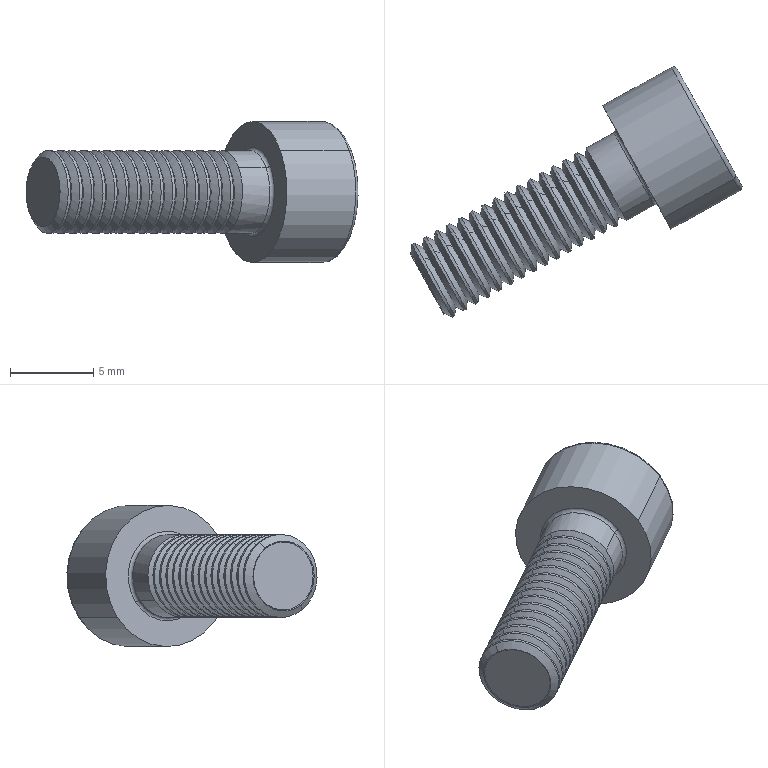Part | STEP file | Socket Head Cap Screw_ISO(ISO 4762 M5 x 20 --- 20S)-8_Valor predeterminado | 1 solid | 119 faces | box 19.995 x 15.067 x 8.5 mm | volume 493.761 mm3 | cone 66 | cylinder 34 | plane 15 | torus 4 | commonest cylinder face diameters 5 x32 8.5 x2